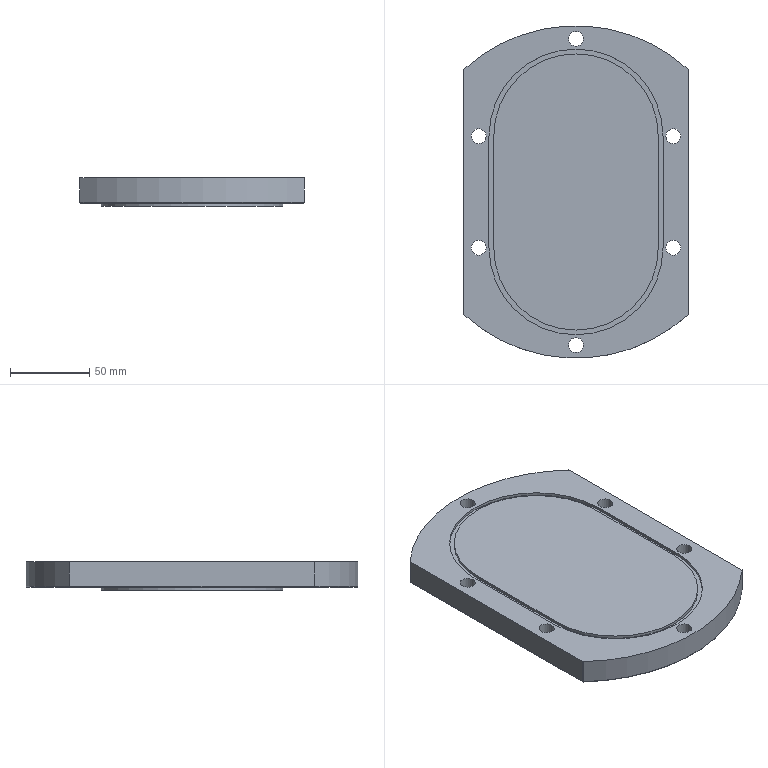NC program | NX | posted with a generic post | part box 142 x 210 x 18 mm
Whole program:
N10 G17 G21 G94 G90
(FLOOR_WALL_COPY_1_COPY , TOOL : D50)
N12 T02 M6
N14 G54
N16 G17 G0 G90 X-67.558 Y67.5 S1200 M3
N18 G43 Z30. H2
N20 Z7.65
N22 G94 G1 Z4.65 F1000.
N24 X-63.246
N26 X63.246 F2000.
N28 G2 X76.103 Y52.58 R92.5
N30 G1 X78.462 Y49.1
N32 X80.108 Y46.249
N34 X82.349 Y42.13
N36 X84.378 Y37.902
N38 X86.19 Y33.578
N40 X87.781 Y29.167
N42 X-87.781
N44 G3 X-92.045 Y-9.167 R92.5
N46 G1 X92.045
N48 G2 X79.373 Y-47.5 R92.5
N50 G1 X-79.373
N52 X-82.849
N54 Z7.65
N56 G0 Z30.
N58 X-67.558 Y67.5
N60 Z7.3
N62 G1 Z4.3 F1000.
N64 X-63.246
N66 X63.246 F2000.
N68 G2 X76.103 Y52.58 R92.5
N70 G1 X78.462 Y49.1
N72 X80.108 Y46.249
N74 X82.349 Y42.13
N76 X84.378 Y37.902
N78 X86.19 Y33.578
N80 X87.781 Y29.167
N82 X-87.781
N84 G3 X-92.045 Y-9.167 R92.5
N86 G1 X92.045
N88 G2 X79.373 Y-47.5 R92.5
N90 G1 X-79.373
N92 X-82.849
N94 Z7.3
N96 G0 Z30.
N98 X-67.558 Y67.5
N100 Z6.95
N102 G1 Z3.95 F1000.
N104 X-63.246
N106 X63.246 F2000.
N108 G2 X76.103 Y52.58 R92.5
N110 G1 X78.462 Y49.1
N112 X80.108 Y46.249
N114 X82.349 Y42.13
N116 X84.378 Y37.902
N118 X86.19 Y33.578
N120 X87.781 Y29.167
N122 X-87.781
N124 G3 X-92.045 Y-9.167 R92.5
N126 G1 X92.045
N128 G2 X79.373 Y-47.5 R92.5
N130 G1 X-79.373
N132 X-82.849
N134 Z6.95
N136 G0 Z30.
N138 X-67.558 Y67.5
N140 Z6.6
N142 G1 Z3.6 F1000.
N144 X-63.246
N146 X63.246 F2000.
N148 G2 X76.103 Y52.58 R92.5
N150 G1 X78.462 Y49.1
N152 X80.108 Y46.249
N154 X82.349 Y42.13
N156 X84.378 Y37.902
N158 X86.19 Y33.578
N160 X87.781 Y29.167
N162 X-87.781
N164 G3 X-92.045 Y-9.167 R92.5
N166 G1 X92.045
N168 G2 X79.373 Y-47.5 R92.5
N170 G1 X-79.373
N172 X-82.849
N174 Z6.6
N176 G0 Z30.
N178 X-67.558 Y67.5
N180 Z6.25
N182 G1 Z3.25 F1000.
N184 X-63.246
N186 X63.246 F2000.
N188 G2 X76.103 Y52.58 R92.5
N190 G1 X78.462 Y49.1
N192 X80.108 Y46.249
N194 X82.349 Y42.13
N196 X84.378 Y37.902
N198 X86.19 Y33.578
N200 X87.781 Y29.167
N202 X-87.781
N204 G3 X-92.045 Y-9.167 R92.5
N206 G1 X92.045
N208 G2 X79.373 Y-47.5 R92.5
N210 G1 X-79.373
N212 X-82.849
N214 Z6.25
N216 G0 Z30.
N218 X-67.558 Y67.5
N220 Z5.9
N222 G1 Z2.9 F1000.
N224 X-63.246
N226 X63.246 F2000.
N228 G2 X76.103 Y52.58 R92.5
N230 G1 X78.462 Y49.1
N232 X80.108 Y46.249
N234 X82.349 Y42.13
N236 X84.378 Y37.902
N238 X86.19 Y33.578
N240 X87.781 Y29.167
N242 X-87.781
N244 G3 X-92.045 Y-9.167 R92.5
N246 G1 X92.045
N248 G2 X79.373 Y-47.5 R92.5
N250 G1 X-79.373
N252 X-82.849
N254 Z5.9
N256 G0 Z30.
N258 X-67.558 Y67.5
N260 Z5.55
N262 G1 Z2.55 F1000.
N264 X-63.246
N266 X63.246 F2000.
N268 G2 X76.103 Y52.58 R92.5
N270 G1 X78.462 Y49.1
N272 X80.108 Y46.249
N274 X82.349 Y42.13
N276 X84.378 Y37.902
N278 X86.19 Y33.578
N280 X87.781 Y29.167
N282 X-87.781
N284 G3 X-92.045 Y-9.167 R92.5
N286 G1 X92.045
N288 G2 X79.373 Y-47.5 R92.5
N290 G1 X-79.373
N292 X-82.849
N294 Z5.55
N296 G0 Z30.
N298 X-67.558 Y67.5
N300 Z5.2
N302 G1 Z2.2 F1000.
N304 X-63.246
N306 X63.246 F2000.
N308 G2 X76.103 Y52.58 R92.5
N310 G1 X78.462 Y49.1
N312 X80.108 Y46.249
N314 X82.349 Y42.13
N316 X84.378 Y37.902
N318 X86.19 Y33.578
N320 X87.781 Y29.167
N322 X-87.781
N324 G3 X-92.045 Y-9.167 R92.5
N326 G1 X92.045
N328 G2 X79.373 Y-47.5 R92.5
N330 G1 X-79.373
N332 X-82.849
N334 Z5.2
N336 G0 Z30.
N338 X-67.558 Y67.5
N340 Z4.85
N342 G1 Z1.85 F1000.
N344 X-63.246
N346 X63.246 F2000.
N348 G2 X76.103 Y52.58 R92.5
N350 G1 X78.462 Y49.1
N352 X80.108 Y46.249
N354 X82.349 Y42.13
N356 X84.378 Y37.902
N358 X86.19 Y33.578
N360 X87.781 Y29.167
N362 X-87.781
N364 G3 X-92.045 Y-9.167 R92.5
N366 G1 X92.045
N368 G2 X79.373 Y-47.5 R92.5
N370 G1 X-79.373
N372 X-82.849
N374 Z4.85
N376 G0 Z30.
N378 X-67.558 Y67.5
N380 Z4.5
N382 G1 Z1.5 F1000.
N384 X-63.246
N386 X63.246 F2000.
N388 G2 X76.103 Y52.58 R92.5
N390 G1 X78.462 Y49.1
N392 X80.108 Y46.249
N394 X82.349 Y42.13
N396 X84.378 Y37.902
N398 X86.19 Y33.578
N400 X87.781 Y29.167
N402 X-87.781
N404 G3 X-92.045 Y-9.167 R92.5
N406 G1 X92.045
N408 G2 X79.373 Y-47.5 R92.5
N410 G1 X-79.373
N412 X-82.849
N414 Z4.5
N416 G0 Z30.
N418 X-67.558 Y67.5
N420 Z4.15
N422 G1 Z1.15 F1000.
N424 X-63.246
N426 X63.246 F2000.
N428 G2 X76.103 Y52.58 R92.5
N430 G1 X78.462 Y49.1
N432 X80.108 Y46.249
N434 X82.349 Y42.13
N436 X84.378 Y37.902
N438 X86.19 Y33.578
N440 X87.781 Y29.167
N442 X-87.781
N444 G3 X-92.045 Y-9.167 R92.5
N446 G1 X92.045
N448 G2 X79.373 Y-47.5 R92.5
N450 G1 X-79.373
N452 X-82.849
N454 Z4.15
N456 G0 Z30.
N458 X-67.558 Y67.5
N460 Z3.8
N462 G1 Z0.8 F1000.
N464 X-63.246
N466 X63.246 F2000.
N468 G2 X76.103 Y52.58 R92.5
N470 G1 X78.462 Y49.1
N472 X80.108 Y46.249
N474 X82.349 Y42.13
N476 X84.378 Y37.902
N478 X86.19 Y33.578
N480 X87.781 Y29.167
N482 X-87.781
N484 G3 X-92.045 Y-9.167 R92.5
N486 G1 X92.045
N488 G2 X79.373 Y-47.5 R92.5
N490 G1 X-79.373
N492 X-82.849
N494 Z3.8
N496 G0 Z30.
N498 X-67.558 Y67.5
N500 Z3.45
N502 G1 Z0.45 F1000.
N504 X-63.246
N506 X63.246 F2000.
N508 G2 X76.103 Y52.58 R92.5
N510 G1 X78.462 Y49.1
N512 X80.108 Y46.249
N514 X82.349 Y42.13
N516 X84.378 Y37.902
N518 X86.19 Y33.578
N520 X87.781 Y29.167
N522 X-87.781
N524 G3 X-92.045 Y-9.167 R92.5
N526 G1 X92.045
N528 G2 X79.373 Y-47.5 R92.5
N530 G1 X-79.373
N532 X-82.849
N534 Z3.45
N536 G0 Z30.
N538 X-67.558 Y67.5
N540 Z3.1
N542 G1 Z0.1 F1000.
N544 X-63.246
N546 X63.246 F2000.
N548 G2 X76.103 Y52.58 R92.5
N550 G1 X78.462 Y49.1
N552 X80.108 Y46.249
N554 X82.349 Y42.13
N556 X84.378 Y37.902
N558 X86.19 Y33.578
N560 X87.781 Y29.167
N562 X-87.781
N564 G3 X-92.045 Y-9.167 R92.5
N566 G1 X92.045
N568 G2 X79.373 Y-47.5 R92.5
N570 G1 X-79.373
N572 X-82.849
N574 Z3.1
N576 G0 Z30.
(FLOOR_WALL_COPY_COPY_COPY , TOOL : D50)
N578 X-67.558 Y67.5 S2500
N580 Z3.
N582 G1 Z0. F1000.
N584 X-63.246
N586 X63.246
N588 G2 X76.103 Y52.58 R92.5
N590 G1 X78.462 Y49.1
N592 X80.108 Y46.249
N594 X82.349 Y42.13
N596 X84.378 Y37.902
N598 X86.19 Y33.578
N600 X87.781 Y29.167
N602 X-87.781
N604 G3 X-92.045 Y-9.167 R92.5
N606 G1 X92.045
N608 G2 X79.373 Y-47.5 R92.5
N610 G1 X-79.373
N612 X-82.849
N614 Z3.
N616 G0 Z30.
N618 M5
(HOLE_MILLING_COPY_COPY , TOOL : D10)
N620 T10 M6
N622 G54
N624 G17 G0 G90 X-35.25 Y61.5 S3000 M3
N626 G43 Z30. H10
N628 Z-1.
N630 G94 G3 X-34.25 Y62.5 R1. F2200.
N632 X-35.25 Y63.5 R1.
N634 X-35.25 Y63.5 Z-1.22 I0. J-2.
N636 X-35.25 Y63.5 Z-1.44 I0. J-2.
N638 X-35.25 Y63.5 Z-1.66 I0. J-2.
N640 X-35.25 Y63.5 Z-1.88 I0. J-2.
N642 X-35.25 Y63.5 Z-2.1 I0. J-2.
N644 X-35.25 Y63.5 Z-2.32 I0. J-2.
N646 X-35.25 Y63.5 Z-2.54 I0. J-2.
N648 X-35.25 Y63.5 Z-2.76 I0. J-2.
N650 X-35.25 Y63.5 Z-2.98 I0. J-2.
N652 X-35.25 Y63.5 Z-3.2 I0. J-2.
N654 X-35.25 Y63.5 Z-3.42 I0. J-2.
N656 X-35.25 Y63.5 Z-3.64 I0. J-2.
N658 X-35.25 Y63.5 Z-3.86 I0. J-2.
N660 X-35.25 Y63.5 Z-4.08 I0. J-2.
N662 X-35.25 Y63.5 Z-4.3 I0. J-2.
N664 X-35.25 Y63.5 Z-4.52 I0. J-2.
N666 X-35.25 Y63.5 Z-4.74 I0. J-2.
N668 X-35.25 Y63.5 Z-4.96 I0. J-2.
N670 X-35.25 Y63.5 Z-5.18 I0. J-2.
N672 X-35.25 Y63.5 Z-5.4 I0. J-2.
N674 X-35.25 Y63.5 Z-5.62 I0. J-2.
N676 X-35.25 Y63.5 Z-5.84 I0. J-2.
N678 X-35.25 Y63.5 Z-6.06 I0. J-2.
N680 X-35.25 Y63.5 Z-6.28 I0. J-2.
N682 X-35.25 Y63.5 Z-6.5 I0. J-2.
N684 X-35.25 Y63.5 Z-6.72 I0. J-2.
N686 X-35.25 Y63.5 Z-6.94 I0. J-2.
N688 X-35.25 Y63.5 Z-7.16 I0. J-2.
N690 X-35.25 Y63.5 Z-7.38 I0. J-2.
N692 X-35.25 Y63.5 Z-7.6 I0. J-2.
N694 X-35.25 Y63.5 Z-7.82 I0. J-2.
N696 X-35.25 Y63.5 Z-8.04 I0. J-2.
N698 X-35.25 Y63.5 Z-8.26 I0. J-2.
N700 X-35.25 Y63.5 Z-8.48 I0. J-2.
N702 X-35.25 Y63.5 Z-8.7 I0. J-2.
N704 X-35.25 Y63.5 Z-8.92 I0. J-2.
N706 X-35.25 Y63.5 Z-9.14 I0. J-2.
N708 X-35.25 Y63.5 Z-9.36 I0. J-2.
N710 X-35.25 Y63.5 Z-9.58 I0. J-2.
N712 X-35.25 Y63.5 Z-9.8 I0. J-2.
N714 X-35.25 Y63.5 Z-10.02 I0. J-2.
N716 X-35.25 Y63.5 Z-10.24 I0. J-2.
N718 X-35.25 Y63.5 Z-10.46 I0. J-2.
N720 X-37.069 Y62.331 Z-10.5 R2.
N722 X-36.081 Y59.681 R2.
N724 X-37.069 Y62.331 R-2.
N726 X-36.575 Y61.006 R1.
N728 X-35.25 Y61.5 R1.
N730 G0 Z30.
N732 X35.25
N734 Z-1.
N736 G3 X36.25 Y62.5 R1.
N738 X35.25 Y63.5 R1.
N740 X35.25 Y63.5 Z-1.22 I0. J-2.
N742 X35.25 Y63.5 Z-1.44 I0. J-2.
N744 X35.25 Y63.5 Z-1.66 I0. J-2.
N746 X35.25 Y63.5 Z-1.88 I0. J-2.
N748 X35.25 Y63.5 Z-2.1 I0. J-2.
N750 X35.25 Y63.5 Z-2.32 I0. J-2.
N752 X35.25 Y63.5 Z-2.54 I0. J-2.
N754 X35.25 Y63.5 Z-2.76 I0. J-2.
N756 X35.25 Y63.5 Z-2.98 I0. J-2.
N758 X35.25 Y63.5 Z-3.2 I0. J-2.
N760 X35.25 Y63.5 Z-3.42 I0. J-2.
N762 X35.25 Y63.5 Z-3.64 I0. J-2.
N764 X35.25 Y63.5 Z-3.86 I0. J-2.
N766 X35.25 Y63.5 Z-4.08 I0. J-2.
N768 X35.25 Y63.5 Z-4.3 I0. J-2.
N770 X35.25 Y63.5 Z-4.52 I0. J-2.
N772 X35.25 Y63.5 Z-4.74 I0. J-2.
N774 X35.25 Y63.5 Z-4.96 I0. J-2.
N776 X35.25 Y63.5 Z-5.18 I0. J-2.
N778 X35.25 Y63.5 Z-5.4 I0. J-2.
N780 X35.25 Y63.5 Z-5.62 I0. J-2.
N782 X35.25 Y63.5 Z-5.84 I0. J-2.
N784 X35.25 Y63.5 Z-6.06 I0. J-2.
N786 X35.25 Y63.5 Z-6.28 I0. J-2.
N788 X35.25 Y63.5 Z-6.5 I0. J-2.
N790 X35.25 Y63.5 Z-6.72 I0. J-2.
N792 X35.25 Y63.5 Z-6.94 I0. J-2.
N794 X35.25 Y63.5 Z-7.16 I0. J-2.
N796 X35.25 Y63.5 Z-7.38 I0. J-2.
N798 X35.25 Y63.5 Z-7.6 I0. J-2.
N800 X35.25 Y63.5 Z-7.82 I0. J-2.
N802 X35.25 Y63.5 Z-8.04 I0. J-2.
N804 X35.25 Y63.5 Z-8.26 I0. J-2.
N806 X35.25 Y63.5 Z-8.48 I0. J-2.
N808 X35.25 Y63.5 Z-8.7 I0. J-2.
N810 X35.25 Y63.5 Z-8.92 I0. J-2.
N812 X35.25 Y63.5 Z-9.14 I0. J-2.
N814 X35.25 Y63.5 Z-9.36 I0. J-2.
N816 X35.25 Y63.5 Z-9.58 I0. J-2.
N818 X35.25 Y63.5 Z-9.8 I0. J-2.
N820 X35.25 Y63.5 Z-10.02 I0. J-2.
N822 X35.25 Y63.5 Z-10.24 I0. J-2.
N824 X35.25 Y63.5 Z-10.46 I0. J-2.
N826 X33.431 Y62.331 Z-10.5 R2.
N828 X34.419 Y59.681 R2.
N830 X33.431 Y62.331 R-2.
N832 X33.925 Y61.006 R1.
N834 X35.25 Y61.5 R1.
N836 G0 Z30.
N838 X96.75 Y0.
N840 Z-1.
N842 G3 X97.75 Y1. R1.
N844 X96.75 Y2. R1.
N846 X96.75 Y2. Z-1.22 I0. J-2.
N848 X96.75 Y2. Z-1.44 I0. J-2.
N850 X96.75 Y2. Z-1.66 I0. J-2.
N852 X96.75 Y2. Z-1.88 I0. J-2.
N854 X96.75 Y2. Z-2.1 I0. J-2.
N856 X96.75 Y2. Z-2.32 I0. J-2.
N858 X96.75 Y2. Z-2.54 I0. J-2.
N860 X96.75 Y2. Z-2.76 I0. J-2.
N862 X96.75 Y2. Z-2.98 I0. J-2.
N864 X96.75 Y2. Z-3.2 I0. J-2.
N866 X96.75 Y2. Z-3.42 I0. J-2.
N868 X96.75 Y2. Z-3.64 I0. J-2.
N870 X96.75 Y2. Z-3.86 I0. J-2.
N872 X96.75 Y2. Z-4.08 I0. J-2.
N874 X96.75 Y2. Z-4.3 I0. J-2.
N876 X96.75 Y2. Z-4.52 I0. J-2.
N878 X96.75 Y2. Z-4.74 I0. J-2.
N880 X96.75 Y2. Z-4.96 I0. J-2.
N882 X96.75 Y2. Z-5.18 I0. J-2.
N884 X96.75 Y2. Z-5.4 I0. J-2.
N886 X96.75 Y2. Z-5.62 I0. J-2.
N888 X96.75 Y2. Z-5.84 I0. J-2.
N890 X96.75 Y2. Z-6.06 I0. J-2.
N892 X96.75 Y2. Z-6.28 I0. J-2.
N894 X96.75 Y2. Z-6.5 I0. J-2.
N896 X96.75 Y2. Z-6.72 I0. J-2.
N898 X96.75 Y2. Z-6.94 I0. J-2.
N900 X96.75 Y2. Z-7.16 I0. J-2.
N902 X96.75 Y2. Z-7.38 I0. J-2.
N904 X96.75 Y2. Z-7.6 I0. J-2.
N906 X96.75 Y2. Z-7.82 I0. J-2.
N908 X96.75 Y2. Z-8.04 I0. J-2.
N910 X96.75 Y2. Z-8.26 I0. J-2.
N912 X96.75 Y2. Z-8.48 I0. J-2.
N914 X96.75 Y2. Z-8.7 I0. J-2.
N916 X96.75 Y2. Z-8.92 I0. J-2.
N918 X96.75 Y2. Z-9.14 I0. J-2.
N920 X96.75 Y2. Z-9.36 I0. J-2.
N922 X96.75 Y2. Z-9.58 I0. J-2.
N924 X96.75 Y2. Z-9.8 I0. J-2.
N926 X96.75 Y2. Z-10.02 I0. J-2.
N928 X96.75 Y2. Z-10.24 I0. J-2.
N930 X96.75 Y2. Z-10.46 I0. J-2.
N932 X94.931 Y0.831 Z-10.5 R2.
N934 X95.919 Y-1.819 R2.
N936 X94.931 Y0.831 R-2.
N938 X95.425 Y-0.494 R1.
N940 X96.75 Y0. R1.
N942 G0 Z30.
N944 X35.25 Y-61.5
N946 Z-1.
N948 G3 X36.25 Y-60.5 R1.
N950 X35.25 Y-59.5 R1.
N952 X35.25 Y-59.5 Z-1.22 I0. J-2.
N954 X35.25 Y-59.5 Z-1.44 I0. J-2.
N956 X35.25 Y-59.5 Z-1.66 I0. J-2.
N958 X35.25 Y-59.5 Z-1.88 I0. J-2.
N960 X35.25 Y-59.5 Z-2.1 I0. J-2.
N962 X35.25 Y-59.5 Z-2.32 I0. J-2.
N964 X35.25 Y-59.5 Z-2.54 I0. J-2.
N966 X35.25 Y-59.5 Z-2.76 I0. J-2.
N968 X35.25 Y-59.5 Z-2.98 I0. J-2.
N970 X35.25 Y-59.5 Z-3.2 I0. J-2.
N972 X35.25 Y-59.5 Z-3.42 I0. J-2.
N974 X35.25 Y-59.5 Z-3.64 I0. J-2.
N976 X35.25 Y-59.5 Z-3.86 I0. J-2.
N978 X35.25 Y-59.5 Z-4.08 I0. J-2.
N980 X35.25 Y-59.5 Z-4.3 I0. J-2.
N982 X35.25 Y-59.5 Z-4.52 I0. J-2.
N984 X35.25 Y-59.5 Z-4.74 I0. J-2.
N986 X35.25 Y-59.5 Z-4.96 I0. J-2.
N988 X35.25 Y-59.5 Z-5.18 I0. J-2.
N990 X35.25 Y-59.5 Z-5.4 I0. J-2.
N992 X35.25 Y-59.5 Z-5.62 I0. J-2.
N994 X35.25 Y-59.5 Z-5.84 I0. J-2.
N996 X35.25 Y-59.5 Z-6.06 I0. J-2.
N998 X35.25 Y-59.5 Z-6.28 I0. J-2.
N1000 X35.25 Y-59.5 Z-6.5 I0. J-2.
N1002 X35.25 Y-59.5 Z-6.72 I0. J-2.
N1004 X35.25 Y-59.5 Z-6.94 I0. J-2.
N1006 X35.25 Y-59.5 Z-7.16 I0. J-2.
N1008 X35.25 Y-59.5 Z-7.38 I0. J-2.
N1010 X35.25 Y-59.5 Z-7.6 I0. J-2.
N1012 X35.25 Y-59.5 Z-7.82 I0. J-2.
N1014 X35.25 Y-59.5 Z-8.04 I0. J-2.
N1016 X35.25 Y-59.5 Z-8.26 I0. J-2.
N1018 X35.25 Y-59.5 Z-8.48 I0. J-2.
N1020 X35.25 Y-59.5 Z-8.7 I0. J-2.
N1022 X35.25 Y-59.5 Z-8.92 I0. J-2.
N1024 X35.25 Y-59.5 Z-9.14 I0. J-2.
N1026 X35.25 Y-59.5 Z-9.36 I0. J-2.
N1028 X35.25 Y-59.5 Z-9.58 I0. J-2.
N1030 X35.25 Y-59.5 Z-9.8 I0. J-2.
N1032 X35.25 Y-59.5 Z-10.02 I0. J-2.
N1034 X35.25 Y-59.5 Z-10.24 I0. J-2.
N1036 X35.25 Y-59.5 Z-10.46 I0. J-2.
N1038 X33.431 Y-60.669 Z-10.5 R2.
N1040 X34.419 Y-63.319 R2.
N1042 X33.431 Y-60.669 R-2.
N1044 X33.925 Y-61.994 R1.
N1046 X35.25 Y-61.5 R1.
N1048 G0 Z30.
N1050 X-35.25
N1052 Z-1.
N1054 G3 X-34.25 Y-60.5 R1.
N1056 X-35.25 Y-59.5 R1.
N1058 X-35.25 Y-59.5 Z-1.22 I0. J-2.
N1060 X-35.25 Y-59.5 Z-1.44 I0. J-2.
N1062 X-35.25 Y-59.5 Z-1.66 I0. J-2.
N1064 X-35.25 Y-59.5 Z-1.88 I0. J-2.
N1066 X-35.25 Y-59.5 Z-2.1 I0. J-2.
N1068 X-35.25 Y-59.5 Z-2.32 I0. J-2.
N1070 X-35.25 Y-59.5 Z-2.54 I0. J-2.
N1072 X-35.25 Y-59.5 Z-2.76 I0. J-2.
N1074 X-35.25 Y-59.5 Z-2.98 I0. J-2.
N1076 X-35.25 Y-59.5 Z-3.2 I0. J-2.
N1078 X-35.25 Y-59.5 Z-3.42 I0. J-2.
N1080 X-35.25 Y-59.5 Z-3.64 I0. J-2.
N1082 X-35.25 Y-59.5 Z-3.86 I0. J-2.
N1084 X-35.25 Y-59.5 Z-4.08 I0. J-2.
N1086 X-35.25 Y-59.5 Z-4.3 I0. J-2.
N1088 X-35.25 Y-59.5 Z-4.52 I0. J-2.
N1090 X-35.25 Y-59.5 Z-4.74 I0. J-2.
N1092 X-35.25 Y-59.5 Z-4.96 I0. J-2.
N1094 X-35.25 Y-59.5 Z-5.18 I0. J-2.
N1096 X-35.25 Y-59.5 Z-5.4 I0. J-2.
N1098 X-35.25 Y-59.5 Z-5.62 I0. J-2.
N1100 X-35.25 Y-59.5 Z-5.84 I0. J-2.
N1102 X-35.25 Y-59.5 Z-6.06 I0. J-2.
N1104 X-35.25 Y-59.5 Z-6.28 I0. J-2.
N1106 X-35.25 Y-59.5 Z-6.5 I0. J-2.
N1108 X-35.25 Y-59.5 Z-6.72 I0. J-2.
N1110 X-35.25 Y-59.5 Z-6.94 I0. J-2.
N1112 X-35.25 Y-59.5 Z-7.16 I0. J-2.
N1114 X-35.25 Y-59.5 Z-7.38 I0. J-2.
N1116 X-35.25 Y-59.5 Z-7.6 I0. J-2.
N1118 X-35.25 Y-59.5 Z-7.82 I0. J-2.
N1120 X-35.25 Y-59.5 Z-8.04 I0. J-2.
N1122 X-35.25 Y-59.5 Z-8.26 I0. J-2.
N1124 X-35.25 Y-59.5 Z-8.48 I0. J-2.
N1126 X-35.25 Y-59.5 Z-8.7 I0. J-2.
N1128 X-35.25 Y-59.5 Z-8.92 I0. J-2.
N1130 X-35.25 Y-59.5 Z-9.14 I0. J-2.
N1132 X-35.25 Y-59.5 Z-9.36 I0. J-2.
N1134 X-35.25 Y-59.5 Z-9.58 I0. J-2.
N1136 X-35.25 Y-59.5 Z-9.8 I0. J-2.
N1138 X-35.25 Y-59.5 Z-10.02 I0. J-2.
N1140 X-35.25 Y-59.5 Z-10.24 I0. J-2.
N1142 X-35.25 Y-59.5 Z-10.46 I0. J-2.
N1144 X-37.069 Y-60.669 Z-10.5 R2.
N1146 X-36.081 Y-63.319 R2.
N1148 X-37.069 Y-60.669 R-2.
N1150 X-36.575 Y-61.994 R1.
N1152 X-35.25 Y-61.5 R1.
N1154 G0 Z30.
N1156 X-96.75 Y0.
N1158 Z-1.
N1160 G3 X-95.75 Y1. R1.
N1162 X-96.75 Y2. R1.
N1164 X-96.75 Y2. Z-1.22 I0. J-2.
N1166 X-96.75 Y2. Z-1.44 I0. J-2.
N1168 X-96.75 Y2. Z-1.66 I0. J-2.
N1170 X-96.75 Y2. Z-1.88 I0. J-2.
N1172 X-96.75 Y2. Z-2.1 I0. J-2.
N1174 X-96.75 Y2. Z-2.32 I0. J-2.
N1176 X-96.75 Y2. Z-2.54 I0. J-2.
N1178 X-96.75 Y2. Z-2.76 I0. J-2.
N1180 X-96.75 Y2. Z-2.98 I0. J-2.
N1182 X-96.75 Y2. Z-3.2 I0. J-2.
N1184 X-96.75 Y2. Z-3.42 I0. J-2.
N1186 X-96.75 Y2. Z-3.64 I0. J-2.
N1188 X-96.75 Y2. Z-3.86 I0. J-2.
N1190 X-96.75 Y2. Z-4.08 I0. J-2.
N1192 X-96.75 Y2. Z-4.3 I0. J-2.
N1194 X-96.75 Y2. Z-4.52 I0. J-2.
N1196 X-96.75 Y2. Z-4.74 I0. J-2.
N1198 X-96.75 Y2. Z-4.96 I0. J-2.
N1200 X-96.75 Y2. Z-5.18 I0. J-2.
N1202 X-96.75 Y2. Z-5.4 I0. J-2.
N1204 X-96.75 Y2. Z-5.62 I0. J-2.
N1206 X-96.75 Y2. Z-5.84 I0. J-2.
N1208 X-96.75 Y2. Z-6.06 I0. J-2.
N1210 X-96.75 Y2. Z-6.28 I0. J-2.
N1212 X-96.75 Y2. Z-6.5 I0. J-2.
N1214 X-96.75 Y2. Z-6.72 I0. J-2.
N1216 X-96.75 Y2. Z-6.94 I0. J-2.
N1218 X-96.75 Y2. Z-7.16 I0. J-2.
N1220 X-96.75 Y2. Z-7.38 I0. J-2.
N1222 X-96.75 Y2. Z-7.6 I0. J-2.
N1224 X-96.75 Y2. Z-7.82 I0. J-2.
N1226 X-96.75 Y2. Z-8.04 I0. J-2.
N1228 X-96.75 Y2. Z-8.26 I0. J-2.
N1230 X-96.75 Y2. Z-8.48 I0. J-2.
N1232 X-96.75 Y2. Z-8.7 I0. J-2.
N1234 X-96.75 Y2. Z-8.92 I0. J-2.
N1236 X-96.75 Y2. Z-9.14 I0. J-2.
N1238 X-96.75 Y2. Z-9.36 I0. J-2.
N1240 X-96.75 Y2. Z-9.58 I0. J-2.
N1242 X-96.75 Y2. Z-9.8 I0. J-2.
N1244 X-96.75 Y2. Z-10.02 I0. J-2.
N1246 X-96.75 Y2. Z-10.24 I0. J-2.
N1248 X-96.75 Y2. Z-10.46 I0. J-2.
N1250 X-98.569 Y0.831 Z-10.5 R2.
N1252 X-97.581 Y-1.819 R2.
N1254 X-98.569 Y0.831 R-2.
N1256 X-98.075 Y-0.494 R1.
N1258 X-96.75 Y0. R1.
N1260 G0 Z30.
N1262 M5
(PLANAR_MILL_COPY_COPY_COPY , TOOL : D6A45)
N1264 T07 M6
N1266 G54
N1268 G17 G0 G90 X-0.766 Y59.157 S7500 M3
N1270 G43 Z30. H7
N1272 Z1.5
N1274 G94 G1 Z-1.5 F1250.
N1276 G3 X0. Y58.8 R1.
N1278 G2 X58.8 Y0. R58.8
N1280 X0. Y58.8 R-58.8
N1282 G3 X0.766 Y59.157 R1.
N1284 G1 Z1.5
N1286 G0 Z30.
(PLANAR_MILL_COPY_COPY_COPY_COPY , TOOL : D6A45)
N1288 X-102.093 Y0.766
N1290 Z-0.5
N1292 G1 Z-3.5
N1294 G3 X-102.45 Y0. R1.
N1296 X-96.75 Y-5.7 R5.7
N1298 X-102.45 Y0. R-5.7
N1300 X-102.093 Y-0.766 R1.
N1302 G1 Z-0.5
N1304 G0 Z30.
N1306 X-36.016 Y-66.843
N1308 Z-0.5
N1310 G1 Z-3.5
N1312 G3 X-35.25 Y-67.2 R1.
N1314 X-29.55 Y-61.5 R5.7
N1316 X-35.25 Y-67.2 R-5.7
N1318 X-34.484 Y-66.843 R1.
N1320 G1 Z-0.5
N1322 G0 Z30.
N1324 X34.484
N1326 Z-0.5
N1328 G1 Z-3.5
N1330 G3 X35.25 Y-67.2 R1.
N1332 X40.95 Y-61.5 R5.7
N1334 X35.25 Y-67.2 R-5.7
N1336 X36.016 Y-66.843 R1.
N1338 G1 Z-0.5
N1340 G0 Z30.
N1342 X0.766 Y-72.657
N1344 Z-0.5
N1346 G1 Z-3.5
N1348 G3 X0. Y-72.3 R1.
N1350 G1 X-77.136
N1352 G2 X-78.465 Y-71.714 R1.8
N1354 X-78.314 Y71.879 R106.3
N1356 X-77.356 Y72.3 R1.3
N1358 G1 X77.136
N1360 G2 X78.465 Y71.714 R1.8
N1362 X78.465 Y-71.714 R106.3
N1364 X77.136 Y-72.3 R1.8
N1366 G1 X0.
N1368 G3 X-0.766 Y-72.657 R1.
N1370 G1 Z-0.5
N1372 G0 Z30.
N1374 X-34.484 Y66.843
N1376 Z-0.5
N1378 G1 Z-3.5
N1380 G3 X-35.25 Y67.2 R1.
N1382 X-40.95 Y61.5 R5.7
N1384 X-35.25 Y67.2 R-5.7
N1386 X-36.016 Y66.843 R1.
N1388 G1 Z-0.5
N1390 G0 Z30.
N1392 X36.016
N1394 Z-0.5
N1396 G1 Z-3.5
N1398 G3 X35.25 Y67.2 R1.
N1400 X29.55 Y61.5 R5.7
N1402 X35.25 Y67.2 R-5.7
N1404 X34.484 Y66.843 R1.
N1406 G1 Z-0.5
N1408 G0 Z30.
N1410 X102.093 Y-0.766
N1412 Z-0.5
N1414 G1 Z-3.5
N1416 G3 X102.45 Y0. R1.
N1418 X96.75 Y5.7 R5.7
N1420 X102.45 Y0. R-5.7
N1422 X102.093 Y0.766 R1.
N1424 G1 Z-0.5
N1426 G0 Z30.
N1428 M5
N1430 M2